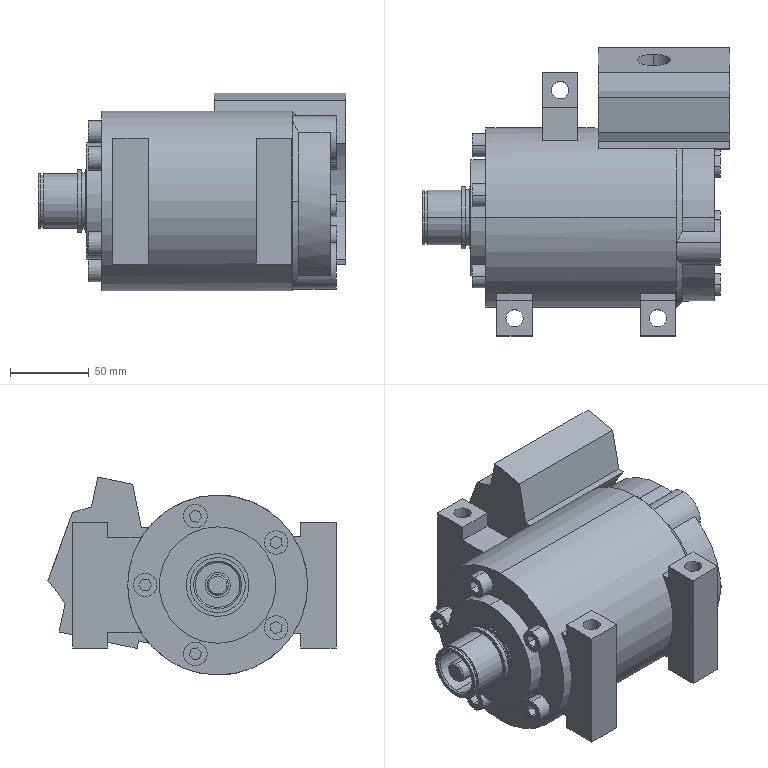Part | STEP file | Market cylinder body | 1 solid | 172 faces | box 195.5 x 183.011 x 125.785 mm | volume 2010849 mm3 | plane 107 | cylinder 58 | cone 7 | commonest cylinder face diameters 15 x10 11 x8 14 x6 29.3 x4 35 x4 40 x4